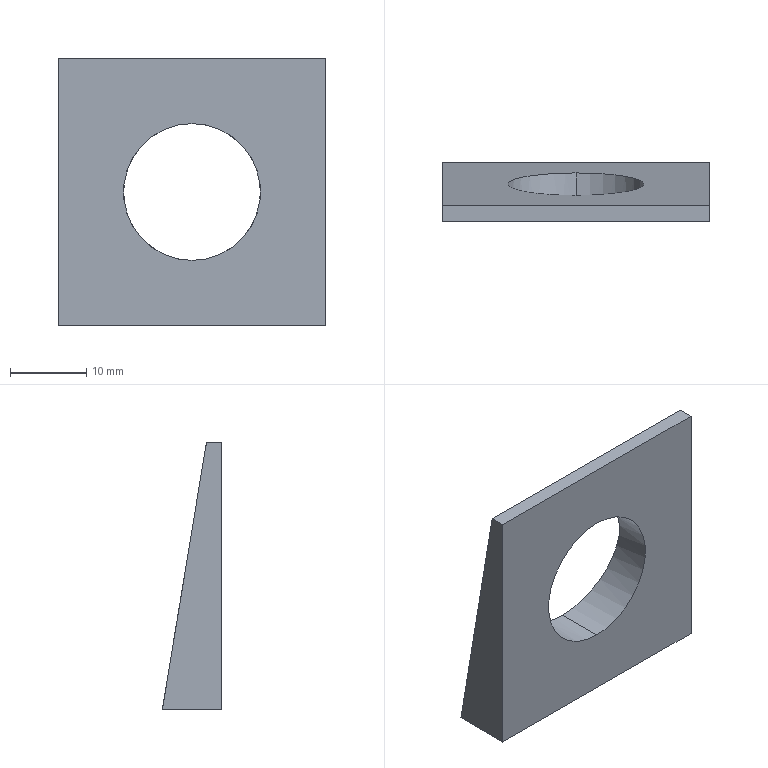Part | STEP file | E3-Square taper washer for I-beam_M16 | 1 solid | 8 faces | box 35 x 7.8 x 35 mm | volume 4756 mm3 | plane 6 | cylinder 2 | commonest cylinder face diameters 18 x2
STEP:
#1=CARTESIAN_POINT('',(0.,0.,0.));
#2=DIRECTION('',(0.,0.,1.));
#3=DIRECTION('',(1.,0.,0.));
#4=AXIS2_PLACEMENT_3D('',#1,#2,#3);
#5=CARTESIAN_POINT('',(0.,3.409,9.));
#6=VERTEX_POINT('',#5);
#7=CARTESIAN_POINT('',(0.,0.,9.));
#8=VERTEX_POINT('',#7);
#9=CARTESIAN_POINT('',(0.,0.,9.));
#10=DIRECTION('',(0.,-1.,0.));
#11=VECTOR('',#10,1.);
#12=LINE('',#9,#11);
#13=CARTESIAN_POINT('',(0.,0.,0.));
#14=DIRECTION('',(0.,-1.,0.));
#15=DIRECTION('',(0.,0.,1.));
#16=AXIS2_PLACEMENT_3D('',#13,#14,#15);
#17=CYLINDRICAL_SURFACE('',#16,9.);
#18=CARTESIAN_POINT('',(6.283,0.));
#19=DIRECTION('',(0.,1.));
#20=VECTOR('',#19,1.);
#21=LINE('',#18,#20);
#22=(GEOMETRIC_REPRESENTATION_CONTEXT(2)PARAMETRIC_REPRESENTATION_CONTEXT()REPRESENTATION_CONTEXT('',''));
#23=DEFINITIONAL_REPRESENTATION('',(#21),#22);
#24=PCURVE('',#17,#23);
#25=CARTESIAN_POINT('',(0.,0.,0.));
#26=DIRECTION('',(0.,-1.,0.));
#27=DIRECTION('',(0.,0.,1.));
#28=AXIS2_PLACEMENT_3D('',#25,#26,#27);
#29=CYLINDRICAL_SURFACE('',#28,9.);
#30=CARTESIAN_POINT('',(0.,0.));
#31=DIRECTION('',(0.,1.));
#32=VECTOR('',#31,1.);
#33=LINE('',#30,#32);
#34=(GEOMETRIC_REPRESENTATION_CONTEXT(2)PARAMETRIC_REPRESENTATION_CONTEXT()REPRESENTATION_CONTEXT('',''));
#35=DEFINITIONAL_REPRESENTATION('',(#33),#34);
#36=PCURVE('',#29,#35);
#37=SURFACE_CURVE('',#12,(#24,#36),.PCURVE_S1.);
#38=EDGE_CURVE('',#6,#8,#37,.T.);
#39=ORIENTED_EDGE('',*,*,#38,.T.);
#40=CARTESIAN_POINT('',(0.,0.,-9.));
#41=VERTEX_POINT('',#40);
#42=CARTESIAN_POINT('',(0.,0.,0.));
#43=DIRECTION('',(0.,1.,0.));
#44=DIRECTION('',(0.,0.,1.));
#45=AXIS2_PLACEMENT_3D('',#42,#43,#44);
#46=CIRCLE('',#45,9.);
#47=CARTESIAN_POINT('',(6.283,0.));
#48=DIRECTION('',(-1.,0.));
#49=VECTOR('',#48,1.);
#50=LINE('',#47,#49);
#51=(GEOMETRIC_REPRESENTATION_CONTEXT(2)PARAMETRIC_REPRESENTATION_CONTEXT()REPRESENTATION_CONTEXT('',''));
#52=DEFINITIONAL_REPRESENTATION('',(#50),#51);
#53=PCURVE('',#17,#52);
#54=CARTESIAN_POINT('',(0.,0.,0.));
#55=DIRECTION('',(0.,1.,0.));
#56=DIRECTION('',(0.,0.,-1.));
#57=AXIS2_PLACEMENT_3D('',#54,#55,#56);
#58=PLANE('',#57);
#59=CARTESIAN_POINT('',(0.,0.));
#60=DIRECTION('',(-1.,0.));
#61=AXIS2_PLACEMENT_2D('',#59,#60);
#62=CIRCLE('',#61,9.);
#63=(GEOMETRIC_REPRESENTATION_CONTEXT(2)PARAMETRIC_REPRESENTATION_CONTEXT()REPRESENTATION_CONTEXT('',''));
#64=DEFINITIONAL_REPRESENTATION('',(#62),#63);
#65=PCURVE('',#58,#64);
#66=SURFACE_CURVE('',#46,(#53,#65),.PCURVE_S1.);
#67=EDGE_CURVE('',#8,#41,#66,.T.);
#68=ORIENTED_EDGE('',*,*,#67,.T.);
#69=CARTESIAN_POINT('',(0.,6.391,-9.));
#70=VERTEX_POINT('',#69);
#71=CARTESIAN_POINT('',(0.,0.,-9.));
#72=DIRECTION('',(0.,-1.,0.));
#73=VECTOR('',#72,1.);
#74=LINE('',#71,#73);
#75=CARTESIAN_POINT('',(3.142,0.));
#76=DIRECTION('',(0.,1.));
#77=VECTOR('',#76,1.);
#78=LINE('',#75,#77);
#79=(GEOMETRIC_REPRESENTATION_CONTEXT(2)PARAMETRIC_REPRESENTATION_CONTEXT()REPRESENTATION_CONTEXT('',''));
#80=DEFINITIONAL_REPRESENTATION('',(#78),#79);
#81=PCURVE('',#17,#80);
#82=CARTESIAN_POINT('',(3.142,0.));
#83=DIRECTION('',(0.,1.));
#84=VECTOR('',#83,1.);
#85=LINE('',#82,#84);
#86=(GEOMETRIC_REPRESENTATION_CONTEXT(2)PARAMETRIC_REPRESENTATION_CONTEXT()REPRESENTATION_CONTEXT('',''));
#87=DEFINITIONAL_REPRESENTATION('',(#85),#86);
#88=PCURVE('',#29,#87);
#89=SURFACE_CURVE('',#74,(#81,#88),.PCURVE_S1.);
#90=EDGE_CURVE('',#70,#41,#89,.T.);
#91=ORIENTED_EDGE('',*,*,#90,.F.);
#92=CARTESIAN_POINT('',(0.,6.391,-9.));
#93=CARTESIAN_POINT('',(18.,6.391,-9.));
#94=CARTESIAN_POINT('',(18.,3.409,9.));
#95=CARTESIAN_POINT('',(0.,3.409,9.));
#96=(BOUNDED_CURVE()B_SPLINE_CURVE(3,(#92,#93,#94,#95),.UNSPECIFIED.,.F.,.F.)B_SPLINE_CURVE_WITH_KNOTS((4,4),(3.142,6.283),.PIECEWISE_BEZIER_KNOTS.)CURVE()GEOMETRIC_REPRESENTATION_ITEM()RATIONAL_B_SPLINE_CURVE((1.,0.3333,0.3333,1.))REPRESENTATION_ITEM(''));
#97=CARTESIAN_POINT('',(3.142,-6.391));
#98=CARTESIAN_POINT('',(3.172,-6.391));
#99=CARTESIAN_POINT('',(3.235,-6.387));
#100=CARTESIAN_POINT('',(3.339,-6.365));
#101=CARTESIAN_POINT('',(3.453,-6.323));
#102=CARTESIAN_POINT('',(3.577,-6.256));
#103=CARTESIAN_POINT('',(3.712,-6.16));
#104=CARTESIAN_POINT('',(3.857,-6.03));
#105=CARTESIAN_POINT('',(4.013,-5.864));
#106=CARTESIAN_POINT('',(4.179,-5.663));
#107=CARTESIAN_POINT('',(4.352,-5.429));
#108=CARTESIAN_POINT('',(4.531,-5.171));
#109=CARTESIAN_POINT('',(4.712,-4.9));
#110=CARTESIAN_POINT('',(4.894,-4.629));
#111=CARTESIAN_POINT('',(5.073,-4.371));
#112=CARTESIAN_POINT('',(5.246,-4.137));
#113=CARTESIAN_POINT('',(5.412,-3.936));
#114=CARTESIAN_POINT('',(5.567,-3.77));
#115=CARTESIAN_POINT('',(5.713,-3.64));
#116=CARTESIAN_POINT('',(5.848,-3.544));
#117=CARTESIAN_POINT('',(5.972,-3.477));
#118=CARTESIAN_POINT('',(6.085,-3.435));
#119=CARTESIAN_POINT('',(6.19,-3.413));
#120=CARTESIAN_POINT('',(6.253,-3.409));
#121=CARTESIAN_POINT('',(6.283,-3.409));
#122=B_SPLINE_CURVE_WITH_KNOTS('',3,(#97,#98,#99,#100,#101,#102,#103,#104,#105,#106,#107,#108,#109,#110,#111,#112,#113,#114,#115,#116,#117,#118,#119,#120,#121),.UNSPECIFIED.,.F.,.F.,(4,1,1,1,1,1,1,1,1,1,1,1,1,1,1,1,1,1,1,1,1,1,4),(3.142,3.284,3.427,3.57,3.713,3.856,3.998,4.141,4.284,4.427,4.57,4.712,4.855,4.998,5.141,5.284,5.426,5.569,5.712,5.855,5.998,6.14,6.283),.QUASI_UNIFORM_KNOTS.);
#123=(GEOMETRIC_REPRESENTATION_CONTEXT(2)PARAMETRIC_REPRESENTATION_CONTEXT()REPRESENTATION_CONTEXT('',''));
#124=DEFINITIONAL_REPRESENTATION('',(#122),#123);
#125=PCURVE('',#17,#124);
#126=CARTESIAN_POINT('',(-17.5,7.8,-17.5));
#127=DIRECTION('',(0.,-0.9865,-0.1635));
#128=DIRECTION('',(0.,-0.1635,0.9865));
#129=AXIS2_PLACEMENT_3D('',#126,#127,#128);
#130=PLANE('',#129);
#131=CARTESIAN_POINT('',(8.616,-17.5));
#132=CARTESIAN_POINT('',(8.616,-35.5));
#133=CARTESIAN_POINT('',(26.861,-35.5));
#134=CARTESIAN_POINT('',(26.861,-17.5));
#135=(BOUNDED_CURVE()B_SPLINE_CURVE(3,(#131,#132,#133,#134),.UNSPECIFIED.,.F.,.F.)B_SPLINE_CURVE_WITH_KNOTS((4,4),(3.142,6.283),.PIECEWISE_BEZIER_KNOTS.)CURVE()GEOMETRIC_REPRESENTATION_ITEM()RATIONAL_B_SPLINE_CURVE((1.,0.3333,0.3333,1.))REPRESENTATION_ITEM(''));
#136=(GEOMETRIC_REPRESENTATION_CONTEXT(2)PARAMETRIC_REPRESENTATION_CONTEXT()REPRESENTATION_CONTEXT('',''));
#137=DEFINITIONAL_REPRESENTATION('',(#135),#136);
#138=PCURVE('',#130,#137);
#139=SURFACE_CURVE('',#96,(#125,#138),.PCURVE_S1.);
#140=EDGE_CURVE('',#70,#6,#139,.T.);
#141=ORIENTED_EDGE('',*,*,#140,.T.);
#142=EDGE_LOOP('',(#39,#68,#91,#141));
#143=FACE_BOUND('',#142,.F.);
#144=ADVANCED_FACE('',(#143),#17,.F.);
#145=CARTESIAN_POINT('',(17.5,2.,17.5));
#146=VERTEX_POINT('',#145);
#147=CARTESIAN_POINT('',(17.5,0.,17.5));
#148=VERTEX_POINT('',#147);
#149=CARTESIAN_POINT('',(17.5,7.8,17.5));
#150=DIRECTION('',(0.,-1.,0.));
#151=VECTOR('',#150,1.);
#152=LINE('',#149,#151);
#153=CARTESIAN_POINT('',(17.5,7.8,17.5));
#154=DIRECTION('',(-1.,0.,0.));
#155=DIRECTION('',(0.,0.,-1.));
#156=AXIS2_PLACEMENT_3D('',#153,#154,#155);
#157=PLANE('',#156);
#158=CARTESIAN_POINT('',(0.,0.));
#159=DIRECTION('',(0.,1.));
#160=VECTOR('',#159,1.);
#161=LINE('',#158,#160);
#162=(GEOMETRIC_REPRESENTATION_CONTEXT(2)PARAMETRIC_REPRESENTATION_CONTEXT()REPRESENTATION_CONTEXT('',''));
#163=DEFINITIONAL_REPRESENTATION('',(#161),#162);
#164=PCURVE('',#157,#163);
#165=CARTESIAN_POINT('',(-17.5,7.8,17.5));
#166=DIRECTION('',(0.,0.,-1.));
#167=DIRECTION('',(1.,0.,0.));
#168=AXIS2_PLACEMENT_3D('',#165,#166,#167);
#169=PLANE('',#168);
#170=CARTESIAN_POINT('',(35.,0.));
#171=DIRECTION('',(0.,1.));
#172=VECTOR('',#171,1.);
#173=LINE('',#170,#172);
#174=(GEOMETRIC_REPRESENTATION_CONTEXT(2)PARAMETRIC_REPRESENTATION_CONTEXT()REPRESENTATION_CONTEXT('',''));
#175=DEFINITIONAL_REPRESENTATION('',(#173),#174);
#176=PCURVE('',#169,#175);
#177=SURFACE_CURVE('',#152,(#164,#176),.PCURVE_S1.);
#178=EDGE_CURVE('',#146,#148,#177,.T.);
#179=ORIENTED_EDGE('',*,*,#178,.T.);
#180=CARTESIAN_POINT('',(17.5,0.,-17.5));
#181=VERTEX_POINT('',#180);
#182=CARTESIAN_POINT('',(17.5,0.,17.5));
#183=DIRECTION('',(0.,0.,1.));
#184=VECTOR('',#183,1.);
#185=LINE('',#182,#184);
#186=CARTESIAN_POINT('',(0.,7.8));
#187=DIRECTION('',(-1.,0.));
#188=VECTOR('',#187,1.);
#189=LINE('',#186,#188);
#190=(GEOMETRIC_REPRESENTATION_CONTEXT(2)PARAMETRIC_REPRESENTATION_CONTEXT()REPRESENTATION_CONTEXT('',''));
#191=DEFINITIONAL_REPRESENTATION('',(#189),#190);
#192=PCURVE('',#157,#191);
#193=CARTESIAN_POINT('',(-17.5,-17.5));
#194=DIRECTION('',(-1.,0.));
#195=VECTOR('',#194,1.);
#196=LINE('',#193,#195);
#197=(GEOMETRIC_REPRESENTATION_CONTEXT(2)PARAMETRIC_REPRESENTATION_CONTEXT()REPRESENTATION_CONTEXT('',''));
#198=DEFINITIONAL_REPRESENTATION('',(#196),#197);
#199=PCURVE('',#58,#198);
#200=SURFACE_CURVE('',#185,(#192,#199),.PCURVE_S1.);
#201=EDGE_CURVE('',#181,#148,#200,.T.);
#202=ORIENTED_EDGE('',*,*,#201,.F.);
#203=CARTESIAN_POINT('',(17.5,7.8,-17.5));
#204=VERTEX_POINT('',#203);
#205=CARTESIAN_POINT('',(17.5,7.8,-17.5));
#206=DIRECTION('',(0.,-1.,0.));
#207=VECTOR('',#206,1.);
#208=LINE('',#205,#207);
#209=CARTESIAN_POINT('',(35.,0.));
#210=DIRECTION('',(0.,1.));
#211=VECTOR('',#210,1.);
#212=LINE('',#209,#211);
#213=(GEOMETRIC_REPRESENTATION_CONTEXT(2)PARAMETRIC_REPRESENTATION_CONTEXT()REPRESENTATION_CONTEXT('',''));
#214=DEFINITIONAL_REPRESENTATION('',(#212),#213);
#215=PCURVE('',#157,#214);
#216=CARTESIAN_POINT('',(-17.5,7.8,-17.5));
#217=DIRECTION('',(0.,0.,1.));
#218=DIRECTION('',(-1.,0.,0.));
#219=AXIS2_PLACEMENT_3D('',#216,#217,#218);
#220=PLANE('',#219);
#221=CARTESIAN_POINT('',(-35.,0.));
#222=DIRECTION('',(0.,1.));
#223=VECTOR('',#222,1.);
#224=LINE('',#221,#223);
#225=(GEOMETRIC_REPRESENTATION_CONTEXT(2)PARAMETRIC_REPRESENTATION_CONTEXT()REPRESENTATION_CONTEXT('',''));
#226=DEFINITIONAL_REPRESENTATION('',(#224),#225);
#227=PCURVE('',#220,#226);
#228=SURFACE_CURVE('',#208,(#215,#227),.PCURVE_S1.);
#229=EDGE_CURVE('',#204,#181,#228,.T.);
#230=ORIENTED_EDGE('',*,*,#229,.F.);
#231=CARTESIAN_POINT('',(17.5,7.8,-17.5));
#232=DIRECTION('',(0.,-0.1635,0.9865));
#233=VECTOR('',#232,1.);
#234=LINE('',#231,#233);
#235=CARTESIAN_POINT('',(35.,0.));
#236=DIRECTION('',(-0.9865,0.1635));
#237=VECTOR('',#236,1.);
#238=LINE('',#235,#237);
#239=(GEOMETRIC_REPRESENTATION_CONTEXT(2)PARAMETRIC_REPRESENTATION_CONTEXT()REPRESENTATION_CONTEXT('',''));
#240=DEFINITIONAL_REPRESENTATION('',(#238),#239);
#241=PCURVE('',#157,#240);
#242=CARTESIAN_POINT('',(0.,-35.));
#243=DIRECTION('',(1.,0.));
#244=VECTOR('',#243,1.);
#245=LINE('',#242,#244);
#246=(GEOMETRIC_REPRESENTATION_CONTEXT(2)PARAMETRIC_REPRESENTATION_CONTEXT()REPRESENTATION_CONTEXT('',''));
#247=DEFINITIONAL_REPRESENTATION('',(#245),#246);
#248=PCURVE('',#130,#247);
#249=SURFACE_CURVE('',#234,(#241,#248),.PCURVE_S1.);
#250=EDGE_CURVE('',#204,#146,#249,.T.);
#251=ORIENTED_EDGE('',*,*,#250,.T.);
#252=EDGE_LOOP('',(#179,#202,#230,#251));
#253=FACE_BOUND('',#252,.T.);
#254=ADVANCED_FACE('',(#253),#157,.F.);
#255=CARTESIAN_POINT('',(-17.5,2.,17.5));
#256=VERTEX_POINT('',#255);
#257=CARTESIAN_POINT('',(-17.5,0.,17.5));
#258=VERTEX_POINT('',#257);
#259=CARTESIAN_POINT('',(-17.5,7.8,17.5));
#260=DIRECTION('',(0.,-1.,0.));
#261=VECTOR('',#260,1.);
#262=LINE('',#259,#261);
#263=CARTESIAN_POINT('',(0.,0.));
#264=DIRECTION('',(0.,1.));
#265=VECTOR('',#264,1.);
#266=LINE('',#263,#265);
#267=(GEOMETRIC_REPRESENTATION_CONTEXT(2)PARAMETRIC_REPRESENTATION_CONTEXT()REPRESENTATION_CONTEXT('',''));
#268=DEFINITIONAL_REPRESENTATION('',(#266),#267);
#269=PCURVE('',#169,#268);
#270=CARTESIAN_POINT('',(-17.5,7.8,17.5));
#271=DIRECTION('',(1.,0.,0.));
#272=DIRECTION('',(0.,0.,1.));
#273=AXIS2_PLACEMENT_3D('',#270,#271,#272);
#274=PLANE('',#273);
#275=CARTESIAN_POINT('',(0.,0.));
#276=DIRECTION('',(0.,1.));
#277=VECTOR('',#276,1.);
#278=LINE('',#275,#277);
#279=(GEOMETRIC_REPRESENTATION_CONTEXT(2)PARAMETRIC_REPRESENTATION_CONTEXT()REPRESENTATION_CONTEXT('',''));
#280=DEFINITIONAL_REPRESENTATION('',(#278),#279);
#281=PCURVE('',#274,#280);
#282=SURFACE_CURVE('',#262,(#269,#281),.PCURVE_S1.);
#283=EDGE_CURVE('',#256,#258,#282,.T.);
#284=ORIENTED_EDGE('',*,*,#283,.T.);
#285=CARTESIAN_POINT('',(-17.5,0.,17.5));
#286=DIRECTION('',(-1.,0.,0.));
#287=VECTOR('',#286,1.);
#288=LINE('',#285,#287);
#289=CARTESIAN_POINT('',(0.,7.8));
#290=DIRECTION('',(-1.,0.));
#291=VECTOR('',#290,1.);
#292=LINE('',#289,#291);
#293=(GEOMETRIC_REPRESENTATION_CONTEXT(2)PARAMETRIC_REPRESENTATION_CONTEXT()REPRESENTATION_CONTEXT('',''));
#294=DEFINITIONAL_REPRESENTATION('',(#292),#293);
#295=PCURVE('',#169,#294);
#296=CARTESIAN_POINT('',(-17.5,17.5));
#297=DIRECTION('',(0.,1.));
#298=VECTOR('',#297,1.);
#299=LINE('',#296,#298);
#300=(GEOMETRIC_REPRESENTATION_CONTEXT(2)PARAMETRIC_REPRESENTATION_CONTEXT()REPRESENTATION_CONTEXT('',''));
#301=DEFINITIONAL_REPRESENTATION('',(#299),#300);
#302=PCURVE('',#58,#301);
#303=SURFACE_CURVE('',#288,(#295,#302),.PCURVE_S1.);
#304=EDGE_CURVE('',#148,#258,#303,.T.);
#305=ORIENTED_EDGE('',*,*,#304,.F.);
#306=ORIENTED_EDGE('',*,*,#178,.F.);
#307=CARTESIAN_POINT('',(-17.5,2.,17.5));
#308=DIRECTION('',(1.,0.,0.));
#309=VECTOR('',#308,1.);
#310=LINE('',#307,#309);
#311=CARTESIAN_POINT('',(0.,5.8));
#312=DIRECTION('',(1.,0.));
#313=VECTOR('',#312,1.);
#314=LINE('',#311,#313);
#315=(GEOMETRIC_REPRESENTATION_CONTEXT(2)PARAMETRIC_REPRESENTATION_CONTEXT()REPRESENTATION_CONTEXT('',''));
#316=DEFINITIONAL_REPRESENTATION('',(#314),#315);
#317=PCURVE('',#169,#316);
#318=CARTESIAN_POINT('',(35.477,0.));
#319=DIRECTION('',(0.,-1.));
#320=VECTOR('',#319,1.);
#321=LINE('',#318,#320);
#322=(GEOMETRIC_REPRESENTATION_CONTEXT(2)PARAMETRIC_REPRESENTATION_CONTEXT()REPRESENTATION_CONTEXT('',''));
#323=DEFINITIONAL_REPRESENTATION('',(#321),#322);
#324=PCURVE('',#130,#323);
#325=SURFACE_CURVE('',#310,(#317,#324),.PCURVE_S1.);
#326=EDGE_CURVE('',#256,#146,#325,.T.);
#327=ORIENTED_EDGE('',*,*,#326,.F.);
#328=EDGE_LOOP('',(#284,#305,#306,#327));
#329=FACE_BOUND('',#328,.T.);
#330=ADVANCED_FACE('',(#329),#169,.F.);
#331=CARTESIAN_POINT('',(-17.5,7.8,-17.5));
#332=VERTEX_POINT('',#331);
#333=CARTESIAN_POINT('',(-17.5,0.,-17.5));
#334=VERTEX_POINT('',#333);
#335=CARTESIAN_POINT('',(-17.5,7.8,-17.5));
#336=DIRECTION('',(0.,-1.,0.));
#337=VECTOR('',#336,1.);
#338=LINE('',#335,#337);
#339=CARTESIAN_POINT('',(-35.,0.));
#340=DIRECTION('',(0.,1.));
#341=VECTOR('',#340,1.);
#342=LINE('',#339,#341);
#343=(GEOMETRIC_REPRESENTATION_CONTEXT(2)PARAMETRIC_REPRESENTATION_CONTEXT()REPRESENTATION_CONTEXT('',''));
#344=DEFINITIONAL_REPRESENTATION('',(#342),#343);
#345=PCURVE('',#274,#344);
#346=CARTESIAN_POINT('',(0.,0.));
#347=DIRECTION('',(0.,1.));
#348=VECTOR('',#347,1.);
#349=LINE('',#346,#348);
#350=(GEOMETRIC_REPRESENTATION_CONTEXT(2)PARAMETRIC_REPRESENTATION_CONTEXT()REPRESENTATION_CONTEXT('',''));
#351=DEFINITIONAL_REPRESENTATION('',(#349),#350);
#352=PCURVE('',#220,#351);
#353=SURFACE_CURVE('',#338,(#345,#352),.PCURVE_S1.);
#354=EDGE_CURVE('',#332,#334,#353,.T.);
#355=ORIENTED_EDGE('',*,*,#354,.T.);
#356=CARTESIAN_POINT('',(-17.5,0.,17.5));
#357=DIRECTION('',(0.,0.,-1.));
#358=VECTOR('',#357,1.);
#359=LINE('',#356,#358);
#360=CARTESIAN_POINT('',(0.,7.8));
#361=DIRECTION('',(-1.,0.));
#362=VECTOR('',#361,1.);
#363=LINE('',#360,#362);
#364=(GEOMETRIC_REPRESENTATION_CONTEXT(2)PARAMETRIC_REPRESENTATION_CONTEXT()REPRESENTATION_CONTEXT('',''));
#365=DEFINITIONAL_REPRESENTATION('',(#363),#364);
#366=PCURVE('',#274,#365);
#367=CARTESIAN_POINT('',(-17.5,17.5));
#368=DIRECTION('',(1.,0.));
#369=VECTOR('',#368,1.);
#370=LINE('',#367,#369);
#371=(GEOMETRIC_REPRESENTATION_CONTEXT(2)PARAMETRIC_REPRESENTATION_CONTEXT()REPRESENTATION_CONTEXT('',''));
#372=DEFINITIONAL_REPRESENTATION('',(#370),#371);
#373=PCURVE('',#58,#372);
#374=SURFACE_CURVE('',#359,(#366,#373),.PCURVE_S1.);
#375=EDGE_CURVE('',#258,#334,#374,.T.);
#376=ORIENTED_EDGE('',*,*,#375,.F.);
#377=ORIENTED_EDGE('',*,*,#283,.F.);
#378=CARTESIAN_POINT('',(-17.5,7.8,-17.5));
#379=DIRECTION('',(0.,-0.1635,0.9865));
#380=VECTOR('',#379,1.);
#381=LINE('',#378,#380);
#382=CARTESIAN_POINT('',(-35.,0.));
#383=DIRECTION('',(0.9865,0.1635));
#384=VECTOR('',#383,1.);
#385=LINE('',#382,#384);
#386=(GEOMETRIC_REPRESENTATION_CONTEXT(2)PARAMETRIC_REPRESENTATION_CONTEXT()REPRESENTATION_CONTEXT('',''));
#387=DEFINITIONAL_REPRESENTATION('',(#385),#386);
#388=PCURVE('',#274,#387);
#389=CARTESIAN_POINT('',(0.,0.));
#390=DIRECTION('',(1.,0.));
#391=VECTOR('',#390,1.);
#392=LINE('',#389,#391);
#393=(GEOMETRIC_REPRESENTATION_CONTEXT(2)PARAMETRIC_REPRESENTATION_CONTEXT()REPRESENTATION_CONTEXT('',''));
#394=DEFINITIONAL_REPRESENTATION('',(#392),#393);
#395=PCURVE('',#130,#394);
#396=SURFACE_CURVE('',#381,(#388,#395),.PCURVE_S1.);
#397=EDGE_CURVE('',#332,#256,#396,.T.);
#398=ORIENTED_EDGE('',*,*,#397,.F.);
#399=EDGE_LOOP('',(#355,#376,#377,#398));
#400=FACE_BOUND('',#399,.T.);
#401=ADVANCED_FACE('',(#400),#274,.F.);
#402=CARTESIAN_POINT('',(-17.5,0.,-17.5));
#403=DIRECTION('',(1.,0.,0.));
#404=VECTOR('',#403,1.);
#405=LINE('',#402,#404);
#406=CARTESIAN_POINT('',(0.,7.8));
#407=DIRECTION('',(-1.,0.));
#408=VECTOR('',#407,1.);
#409=LINE('',#406,#408);
#410=(GEOMETRIC_REPRESENTATION_CONTEXT(2)PARAMETRIC_REPRESENTATION_CONTEXT()REPRESENTATION_CONTEXT('',''));
#411=DEFINITIONAL_REPRESENTATION('',(#409),#410);
#412=PCURVE('',#220,#411);
#413=CARTESIAN_POINT('',(17.5,17.5));
#414=DIRECTION('',(0.,-1.));
#415=VECTOR('',#414,1.);
#416=LINE('',#413,#415);
#417=(GEOMETRIC_REPRESENTATION_CONTEXT(2)PARAMETRIC_REPRESENTATION_CONTEXT()REPRESENTATION_CONTEXT('',''));
#418=DEFINITIONAL_REPRESENTATION('',(#416),#417);
#419=PCURVE('',#58,#418);
#420=SURFACE_CURVE('',#405,(#412,#419),.PCURVE_S1.);
#421=EDGE_CURVE('',#334,#181,#420,.T.);
#422=ORIENTED_EDGE('',*,*,#421,.F.);
#423=ORIENTED_EDGE('',*,*,#354,.F.);
#424=CARTESIAN_POINT('',(-17.5,7.8,-17.5));
#425=DIRECTION('',(1.,0.,0.));
#426=VECTOR('',#425,1.);
#427=LINE('',#424,#426);
#428=CARTESIAN_POINT('',(0.,0.));
#429=DIRECTION('',(-1.,0.));
#430=VECTOR('',#429,1.);
#431=LINE('',#428,#430);
#432=(GEOMETRIC_REPRESENTATION_CONTEXT(2)PARAMETRIC_REPRESENTATION_CONTEXT()REPRESENTATION_CONTEXT('',''));
#433=DEFINITIONAL_REPRESENTATION('',(#431),#432);
#434=PCURVE('',#220,#433);
#435=CARTESIAN_POINT('',(0.,0.));
#436=DIRECTION('',(0.,-1.));
#437=VECTOR('',#436,1.);
#438=LINE('',#435,#437);
#439=(GEOMETRIC_REPRESENTATION_CONTEXT(2)PARAMETRIC_REPRESENTATION_CONTEXT()REPRESENTATION_CONTEXT('',''));
#440=DEFINITIONAL_REPRESENTATION('',(#438),#439);
#441=PCURVE('',#130,#440);
#442=SURFACE_CURVE('',#427,(#434,#441),.PCURVE_S1.);
#443=EDGE_CURVE('',#332,#204,#442,.T.);
#444=ORIENTED_EDGE('',*,*,#443,.T.);
#445=ORIENTED_EDGE('',*,*,#229,.T.);
#446=EDGE_LOOP('',(#422,#423,#444,#445));
#447=FACE_BOUND('',#446,.T.);
#448=ADVANCED_FACE('',(#447),#220,.F.);
#449=ORIENTED_EDGE('',*,*,#67,.T.);
#450=CARTESIAN_POINT('',(0.,0.,0.));
#451=DIRECTION('',(0.,1.,0.));
#452=DIRECTION('',(0.,0.,1.));
#453=AXIS2_PLACEMENT_3D('',#450,#451,#452);
#454=CIRCLE('',#453,9.);
#455=CARTESIAN_POINT('',(0.,0.));
#456=DIRECTION('',(-1.,0.));
#457=AXIS2_PLACEMENT_2D('',#455,#456);
#458=CIRCLE('',#457,9.);
#459=(GEOMETRIC_REPRESENTATION_CONTEXT(2)PARAMETRIC_REPRESENTATION_CONTEXT()REPRESENTATION_CONTEXT('',''));
#460=DEFINITIONAL_REPRESENTATION('',(#458),#459);
#461=PCURVE('',#58,#460);
#462=CARTESIAN_POINT('',(6.283,0.));
#463=DIRECTION('',(-1.,0.));
#464=VECTOR('',#463,1.);
#465=LINE('',#462,#464);
#466=(GEOMETRIC_REPRESENTATION_CONTEXT(2)PARAMETRIC_REPRESENTATION_CONTEXT()REPRESENTATION_CONTEXT('',''));
#467=DEFINITIONAL_REPRESENTATION('',(#465),#466);
#468=PCURVE('',#29,#467);
#469=SURFACE_CURVE('',#454,(#461,#468),.PCURVE_S1.);
#470=EDGE_CURVE('',#41,#8,#469,.T.);
#471=ORIENTED_EDGE('',*,*,#470,.T.);
#472=EDGE_LOOP('',(#449,#471));
#473=FACE_BOUND('',#472,.T.);
#474=ORIENTED_EDGE('',*,*,#201,.T.);
#475=ORIENTED_EDGE('',*,*,#304,.T.);
#476=ORIENTED_EDGE('',*,*,#375,.T.);
#477=ORIENTED_EDGE('',*,*,#421,.T.);
#478=EDGE_LOOP('',(#474,#475,#476,#477));
#479=FACE_BOUND('',#478,.T.);
#480=ADVANCED_FACE('',(#473,#479),#58,.F.);
#481=ORIENTED_EDGE('',*,*,#470,.T.);
#482=ORIENTED_EDGE('',*,*,#38,.F.);
#483=CARTESIAN_POINT('',(0.,3.409,9.));
#484=CARTESIAN_POINT('',(-18.,3.409,9.));
#485=CARTESIAN_POINT('',(-18.,6.391,-9.));
#486=CARTESIAN_POINT('',(0.,6.391,-9.));
#487=(BOUNDED_CURVE()B_SPLINE_CURVE(3,(#483,#484,#485,#486),.UNSPECIFIED.,.F.,.F.)B_SPLINE_CURVE_WITH_KNOTS((4,4),(0.,3.142),.PIECEWISE_BEZIER_KNOTS.)CURVE()GEOMETRIC_REPRESENTATION_ITEM()RATIONAL_B_SPLINE_CURVE((1.,0.3333,0.3333,1.))REPRESENTATION_ITEM(''));
#488=CARTESIAN_POINT('',(0.,-3.409));
#489=CARTESIAN_POINT('',(0.0303,-3.409));
#490=CARTESIAN_POINT('',(0.09367,-3.413));
#491=CARTESIAN_POINT('',(0.1977,-3.435));
#492=CARTESIAN_POINT('',(0.3115,-3.477));
#493=CARTESIAN_POINT('',(0.4356,-3.544));
#494=CARTESIAN_POINT('',(0.5703,-3.64));
#495=CARTESIAN_POINT('',(0.7158,-3.77));
#496=CARTESIAN_POINT('',(0.8717,-3.936));
#497=CARTESIAN_POINT('',(1.037,-4.137));
#498=CARTESIAN_POINT('',(1.21,-4.371));
#499=CARTESIAN_POINT('',(1.389,-4.629));
#500=CARTESIAN_POINT('',(1.571,-4.9));
#501=CARTESIAN_POINT('',(1.753,-5.171));
#502=CARTESIAN_POINT('',(1.931,-5.429));
#503=CARTESIAN_POINT('',(2.105,-5.663));
#504=CARTESIAN_POINT('',(2.27,-5.864));
#505=CARTESIAN_POINT('',(2.426,-6.03));
#506=CARTESIAN_POINT('',(2.571,-6.16));
#507=CARTESIAN_POINT('',(2.706,-6.256));
#508=CARTESIAN_POINT('',(2.83,-6.323));
#509=CARTESIAN_POINT('',(2.944,-6.365));
#510=CARTESIAN_POINT('',(3.048,-6.387));
#511=CARTESIAN_POINT('',(3.111,-6.391));
#512=CARTESIAN_POINT('',(3.142,-6.391));
#513=B_SPLINE_CURVE_WITH_KNOTS('',3,(#488,#489,#490,#491,#492,#493,#494,#495,#496,#497,#498,#499,#500,#501,#502,#503,#504,#505,#506,#507,#508,#509,#510,#511,#512),.UNSPECIFIED.,.F.,.F.,(4,1,1,1,1,1,1,1,1,1,1,1,1,1,1,1,1,1,1,1,1,1,4),(0.,0.1428,0.2856,0.4284,0.5712,0.714,0.8568,0.9996,1.142,1.285,1.428,1.571,1.714,1.856,1.999,2.142,2.285,2.428,2.57,2.713,2.856,2.999,3.142),.QUASI_UNIFORM_KNOTS.);
#514=(GEOMETRIC_REPRESENTATION_CONTEXT(2)PARAMETRIC_REPRESENTATION_CONTEXT()REPRESENTATION_CONTEXT('',''));
#515=DEFINITIONAL_REPRESENTATION('',(#513),#514);
#516=PCURVE('',#29,#515);
#517=CARTESIAN_POINT('',(26.861,-17.5));
#518=CARTESIAN_POINT('',(26.861,0.5));
#519=CARTESIAN_POINT('',(8.616,0.5));
#520=CARTESIAN_POINT('',(8.616,-17.5));
#521=(BOUNDED_CURVE()B_SPLINE_CURVE(3,(#517,#518,#519,#520),.UNSPECIFIED.,.F.,.F.)B_SPLINE_CURVE_WITH_KNOTS((4,4),(0.,3.142),.PIECEWISE_BEZIER_KNOTS.)CURVE()GEOMETRIC_REPRESENTATION_ITEM()RATIONAL_B_SPLINE_CURVE((1.,0.3333,0.3333,1.))REPRESENTATION_ITEM(''));
#522=(GEOMETRIC_REPRESENTATION_CONTEXT(2)PARAMETRIC_REPRESENTATION_CONTEXT()REPRESENTATION_CONTEXT('',''));
#523=DEFINITIONAL_REPRESENTATION('',(#521),#522);
#524=PCURVE('',#130,#523);
#525=SURFACE_CURVE('',#487,(#516,#524),.PCURVE_S1.);
#526=EDGE_CURVE('',#6,#70,#525,.T.);
#527=ORIENTED_EDGE('',*,*,#526,.T.);
#528=ORIENTED_EDGE('',*,*,#90,.T.);
#529=EDGE_LOOP('',(#481,#482,#527,#528));
#530=FACE_BOUND('',#529,.F.);
#531=ADVANCED_FACE('',(#530),#29,.F.);
#532=ORIENTED_EDGE('',*,*,#326,.T.);
#533=ORIENTED_EDGE('',*,*,#250,.F.);
#534=ORIENTED_EDGE('',*,*,#443,.F.);
#535=ORIENTED_EDGE('',*,*,#397,.T.);
#536=EDGE_LOOP('',(#532,#533,#534,#535));
#537=FACE_BOUND('',#536,.T.);
#538=ORIENTED_EDGE('',*,*,#526,.T.);
#539=ORIENTED_EDGE('',*,*,#140,.T.);
#540=EDGE_LOOP('',(#538,#539));
#541=FACE_BOUND('',#540,.T.);
#542=ADVANCED_FACE('',(#537,#541),#130,.F.);
#543=CLOSED_SHELL('',(#144,#254,#330,#401,#448,#480,#531,#542));
#544=MANIFOLD_SOLID_BREP('',#543);
#545=(LENGTH_UNIT()NAMED_UNIT(*)SI_UNIT(.MILLI.,.METRE.));
#546=UNCERTAINTY_MEASURE_WITH_UNIT(LENGTH_MEASURE(0.0000001),#545,'','');
#547=(NAMED_UNIT(*)PLANE_ANGLE_UNIT()SI_UNIT($,.RADIAN.));
#548=(NAMED_UNIT(*)SI_UNIT($,.STERADIAN.)SOLID_ANGLE_UNIT());
#549=(GEOMETRIC_REPRESENTATION_CONTEXT(3)GLOBAL_UNCERTAINTY_ASSIGNED_CONTEXT((#546))GLOBAL_UNIT_ASSIGNED_CONTEXT((#545,#547,#548))REPRESENTATION_CONTEXT('',''));
#550=ADVANCED_BREP_SHAPE_REPRESENTATION('',(#4,#544),#549);